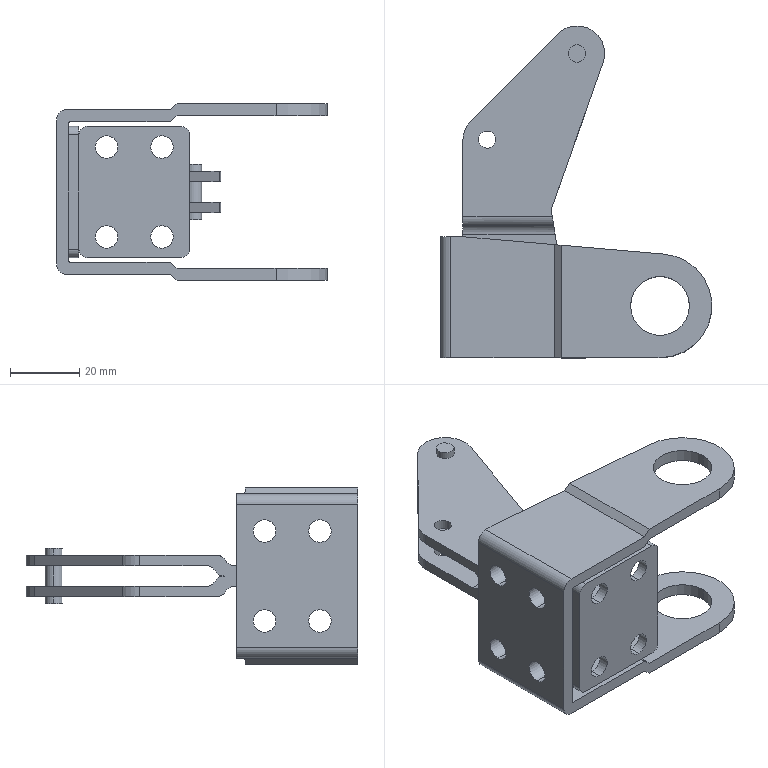Part | STEP file | Sceond_200_APVM -1 | 1 solid | 106 faces | box 78.4 x 96 x 51 mm | volume 41940 mm3 | cylinder 60 | plane 46 | commonest cylinder face diameters 5 x18 6.5 x16 6 x10 16 x4 17 x4 30 x4